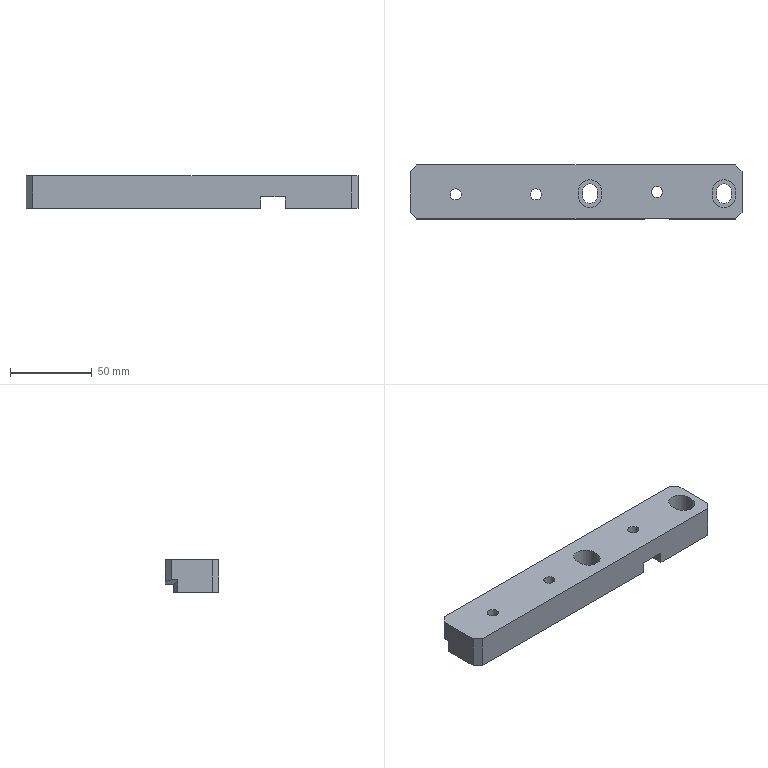Part | NX | features 20 2 | 1 solid | 43 faces | box 203 x 33 x 20 mm | volume 116194 mm3 | plane 32 | cylinder 11 | commonest cylinder face diameters 9 x4 14 x4 6.8 x3
STEP:
#1=CARTESIAN_POINT('',(39.002,-433.5,16.5));
#2=VERTEX_POINT('',#1);
#3=CARTESIAN_POINT('',(25.002,-433.5,16.5));
#4=VERTEX_POINT('',#3);
#5=CARTESIAN_POINT('',(32.002,-433.5,16.5));
#6=DIRECTION('',(0.,0.,1.));
#7=DIRECTION('',(1.,0.,0.));
#8=AXIS2_PLACEMENT_3D('',#5,#6,#7);
#9=CIRCLE('',#8,7.);
#10=EDGE_CURVE('',#2,#4,#9,.T.);
#11=ORIENTED_EDGE('',*,*,#10,.F.);
#12=CARTESIAN_POINT('',(39.002,-436.5,16.5));
#13=VERTEX_POINT('',#12);
#14=CARTESIAN_POINT('',(39.002,-450.5,16.5));
#15=DIRECTION('',(0.,1.,0.));
#16=VECTOR('',#15,1000.);
#17=LINE('',#14,#16);
#18=EDGE_CURVE('',#13,#2,#17,.T.);
#19=ORIENTED_EDGE('',*,*,#18,.F.);
#20=CARTESIAN_POINT('',(25.002,-436.5,16.5));
#21=VERTEX_POINT('',#20);
#22=CARTESIAN_POINT('',(32.002,-436.5,16.5));
#23=DIRECTION('',(0.,0.,1.));
#24=DIRECTION('',(1.,0.,0.));
#25=AXIS2_PLACEMENT_3D('',#22,#23,#24);
#26=CIRCLE('',#25,7.);
#27=EDGE_CURVE('',#21,#13,#26,.T.);
#28=ORIENTED_EDGE('',*,*,#27,.F.);
#29=CARTESIAN_POINT('',(25.002,-450.5,16.5));
#30=DIRECTION('',(0.,-1.,0.));
#31=VECTOR('',#30,1000.);
#32=LINE('',#29,#31);
#33=EDGE_CURVE('',#4,#21,#32,.T.);
#34=ORIENTED_EDGE('',*,*,#33,.F.);
#35=EDGE_LOOP('',(#11,#19,#28,#34));
#36=FACE_BOUND('',#35,.T.);
#37=CARTESIAN_POINT('',(39.002,-417.5,16.5));
#38=VERTEX_POINT('',#37);
#39=CARTESIAN_POINT('',(-155.998,-417.5,16.5));
#40=VERTEX_POINT('',#39);
#41=CARTESIAN_POINT('',(-45.998,-417.5,16.5));
#42=DIRECTION('',(-1.,0.,0.));
#43=VECTOR('',#42,1000.);
#44=LINE('',#41,#43);
#45=EDGE_CURVE('',#38,#40,#44,.T.);
#46=ORIENTED_EDGE('',*,*,#45,.T.);
#47=CARTESIAN_POINT('',(-159.998,-421.5,16.5));
#48=VERTEX_POINT('',#47);
#49=CARTESIAN_POINT('',(-159.998,-421.5,16.5));
#50=DIRECTION('',(-0.7071,-0.7071,0.));
#51=VECTOR('',#50,1000.);
#52=LINE('',#49,#51);
#53=EDGE_CURVE('',#40,#48,#52,.T.);
#54=ORIENTED_EDGE('',*,*,#53,.T.);
#55=CARTESIAN_POINT('',(-159.998,-446.5,16.5));
#56=VERTEX_POINT('',#55);
#57=CARTESIAN_POINT('',(-159.998,-417.5,16.5));
#58=DIRECTION('',(0.,-1.,0.));
#59=VECTOR('',#58,1000.);
#60=LINE('',#57,#59);
#61=EDGE_CURVE('',#48,#56,#60,.T.);
#62=ORIENTED_EDGE('',*,*,#61,.T.);
#63=CARTESIAN_POINT('',(-155.998,-450.5,16.5));
#64=VERTEX_POINT('',#63);
#65=CARTESIAN_POINT('',(-155.998,-450.5,16.5));
#66=DIRECTION('',(0.7071,-0.7071,0.));
#67=VECTOR('',#66,1000.);
#68=LINE('',#65,#67);
#69=EDGE_CURVE('',#56,#64,#68,.T.);
#70=ORIENTED_EDGE('',*,*,#69,.T.);
#71=CARTESIAN_POINT('',(39.002,-450.5,16.5));
#72=VERTEX_POINT('',#71);
#73=CARTESIAN_POINT('',(-125.998,-450.5,16.5));
#74=DIRECTION('',(1.,0.,0.));
#75=VECTOR('',#74,1000.);
#76=LINE('',#73,#75);
#77=EDGE_CURVE('',#64,#72,#76,.T.);
#78=ORIENTED_EDGE('',*,*,#77,.T.);
#79=CARTESIAN_POINT('',(43.002,-446.5,16.5));
#80=VERTEX_POINT('',#79);
#81=CARTESIAN_POINT('',(43.002,-446.5,16.5));
#82=DIRECTION('',(0.7071,0.7071,0.));
#83=VECTOR('',#82,1000.);
#84=LINE('',#81,#83);
#85=EDGE_CURVE('',#72,#80,#84,.T.);
#86=ORIENTED_EDGE('',*,*,#85,.T.);
#87=CARTESIAN_POINT('',(43.002,-421.5,16.5));
#88=VERTEX_POINT('',#87);
#89=CARTESIAN_POINT('',(43.002,-450.5,16.5));
#90=DIRECTION('',(0.,1.,0.));
#91=VECTOR('',#90,1000.);
#92=LINE('',#89,#91);
#93=EDGE_CURVE('',#80,#88,#92,.T.);
#94=ORIENTED_EDGE('',*,*,#93,.T.);
#95=CARTESIAN_POINT('',(39.002,-417.5,16.5));
#96=DIRECTION('',(-0.7071,0.7071,0.));
#97=VECTOR('',#96,1000.);
#98=LINE('',#95,#97);
#99=EDGE_CURVE('',#88,#38,#98,.T.);
#100=ORIENTED_EDGE('',*,*,#99,.T.);
#101=EDGE_LOOP('',(#46,#54,#62,#70,#78,#86,#94,#100));
#102=FACE_BOUND('',#101,.T.);
#103=CARTESIAN_POINT('',(-42.998,-436.5,16.5));
#104=VERTEX_POINT('',#103);
#105=CARTESIAN_POINT('',(-42.998,-433.5,16.5));
#106=VERTEX_POINT('',#105);
#107=CARTESIAN_POINT('',(-42.998,-450.5,16.5));
#108=DIRECTION('',(0.,1.,0.));
#109=VECTOR('',#108,1000.);
#110=LINE('',#107,#109);
#111=EDGE_CURVE('',#104,#106,#110,.T.);
#112=ORIENTED_EDGE('',*,*,#111,.F.);
#113=CARTESIAN_POINT('',(-56.998,-436.5,16.5));
#114=VERTEX_POINT('',#113);
#115=CARTESIAN_POINT('',(-49.998,-436.5,16.5));
#116=DIRECTION('',(0.,0.,1.));
#117=DIRECTION('',(1.,0.,0.));
#118=AXIS2_PLACEMENT_3D('',#115,#116,#117);
#119=CIRCLE('',#118,7.);
#120=EDGE_CURVE('',#114,#104,#119,.T.);
#121=ORIENTED_EDGE('',*,*,#120,.F.);
#122=CARTESIAN_POINT('',(-56.998,-433.5,16.5));
#123=VERTEX_POINT('',#122);
#124=CARTESIAN_POINT('',(-56.998,-450.5,16.5));
#125=DIRECTION('',(0.,-1.,0.));
#126=VECTOR('',#125,1000.);
#127=LINE('',#124,#126);
#128=EDGE_CURVE('',#123,#114,#127,.T.);
#129=ORIENTED_EDGE('',*,*,#128,.F.);
#130=CARTESIAN_POINT('',(-49.998,-433.5,16.5));
#131=DIRECTION('',(0.,0.,1.));
#132=DIRECTION('',(1.,0.,0.));
#133=AXIS2_PLACEMENT_3D('',#130,#131,#132);
#134=CIRCLE('',#133,7.);
#135=EDGE_CURVE('',#106,#123,#134,.T.);
#136=ORIENTED_EDGE('',*,*,#135,.F.);
#137=EDGE_LOOP('',(#112,#121,#129,#136));
#138=FACE_BOUND('',#137,.T.);
#139=CARTESIAN_POINT('',(-79.598,-435.5,16.5));
#140=VERTEX_POINT('',#139);
#141=CARTESIAN_POINT('',(-82.998,-435.5,16.5));
#142=DIRECTION('',(0.,0.,1.));
#143=DIRECTION('',(1.,0.,0.));
#144=AXIS2_PLACEMENT_3D('',#141,#142,#143);
#145=CIRCLE('',#144,3.4);
#146=EDGE_CURVE('',#140,#140,#145,.T.);
#147=ORIENTED_EDGE('',*,*,#146,.F.);
#148=EDGE_LOOP('',(#147));
#149=FACE_BOUND('',#148,.T.);
#150=CARTESIAN_POINT('',(-128.598,-435.5,16.5));
#151=VERTEX_POINT('',#150);
#152=CARTESIAN_POINT('',(-131.998,-435.5,16.5));
#153=DIRECTION('',(0.,0.,1.));
#154=DIRECTION('',(1.,0.,0.));
#155=AXIS2_PLACEMENT_3D('',#152,#153,#154);
#156=CIRCLE('',#155,3.4);
#157=EDGE_CURVE('',#151,#151,#156,.T.);
#158=ORIENTED_EDGE('',*,*,#157,.F.);
#159=EDGE_LOOP('',(#158));
#160=FACE_BOUND('',#159,.T.);
#161=CARTESIAN_POINT('',(-5.598,-434.,16.5));
#162=VERTEX_POINT('',#161);
#163=CARTESIAN_POINT('',(-8.998,-434.,16.5));
#164=DIRECTION('',(0.,0.,-1.));
#165=DIRECTION('',(1.,0.,0.));
#166=AXIS2_PLACEMENT_3D('',#163,#164,#165);
#167=CIRCLE('',#166,3.4);
#168=EDGE_CURVE('',#162,#162,#167,.T.);
#169=ORIENTED_EDGE('',*,*,#168,.T.);
#170=EDGE_LOOP('',(#169));
#171=FACE_BOUND('',#170,.T.);
#172=CARTESIAN_POINT('',(-45.998,-450.5,16.5));
#173=DIRECTION('',(0.,0.,1.));
#174=DIRECTION('',(-1.,0.,0.));
#175=AXIS2_PLACEMENT_3D('',#172,#173,#174);
#176=PLANE('',#175);
#177=ADVANCED_FACE('',(#36,#102,#138,#149,#160,#171),#176,.T.);
#178=CARTESIAN_POINT('',(-45.498,-433.5,1.5));
#179=VERTEX_POINT('',#178);
#180=CARTESIAN_POINT('',(-45.498,-436.5,1.5));
#181=VERTEX_POINT('',#180);
#182=CARTESIAN_POINT('',(-45.498,-432.5,1.5));
#183=DIRECTION('',(0.,-1.,0.));
#184=VECTOR('',#183,1000.);
#185=LINE('',#182,#184);
#186=EDGE_CURVE('',#179,#181,#185,.T.);
#187=ORIENTED_EDGE('',*,*,#186,.T.);
#188=CARTESIAN_POINT('',(-54.498,-436.5,1.5));
#189=VERTEX_POINT('',#188);
#190=CARTESIAN_POINT('',(-49.998,-436.5,1.5));
#191=DIRECTION('',(0.,0.,-1.));
#192=DIRECTION('',(-1.,0.,0.));
#193=AXIS2_PLACEMENT_3D('',#190,#191,#192);
#194=CIRCLE('',#193,4.5);
#195=EDGE_CURVE('',#181,#189,#194,.T.);
#196=ORIENTED_EDGE('',*,*,#195,.T.);
#197=CARTESIAN_POINT('',(-54.498,-433.5,1.5));
#198=VERTEX_POINT('',#197);
#199=CARTESIAN_POINT('',(-54.498,-439.5,1.5));
#200=DIRECTION('',(0.,1.,0.));
#201=VECTOR('',#200,1000.);
#202=LINE('',#199,#201);
#203=EDGE_CURVE('',#189,#198,#202,.T.);
#204=ORIENTED_EDGE('',*,*,#203,.T.);
#205=CARTESIAN_POINT('',(-49.998,-433.5,1.5));
#206=DIRECTION('',(0.,0.,-1.));
#207=DIRECTION('',(-1.,0.,0.));
#208=AXIS2_PLACEMENT_3D('',#205,#206,#207);
#209=CIRCLE('',#208,4.5);
#210=EDGE_CURVE('',#198,#179,#209,.T.);
#211=ORIENTED_EDGE('',*,*,#210,.T.);
#212=EDGE_LOOP('',(#187,#196,#204,#211));
#213=FACE_BOUND('',#212,.T.);
#214=CARTESIAN_POINT('',(-42.998,-433.5,1.5));
#215=VERTEX_POINT('',#214);
#216=CARTESIAN_POINT('',(-56.998,-433.5,1.5));
#217=VERTEX_POINT('',#216);
#218=CARTESIAN_POINT('',(-49.998,-433.5,1.5));
#219=DIRECTION('',(0.,0.,1.));
#220=DIRECTION('',(1.,0.,0.));
#221=AXIS2_PLACEMENT_3D('',#218,#219,#220);
#222=CIRCLE('',#221,7.);
#223=EDGE_CURVE('',#215,#217,#222,.T.);
#224=ORIENTED_EDGE('',*,*,#223,.T.);
#225=CARTESIAN_POINT('',(-56.998,-436.5,1.5));
#226=VERTEX_POINT('',#225);
#227=CARTESIAN_POINT('',(-56.998,-432.5,1.5));
#228=DIRECTION('',(0.,-1.,0.));
#229=VECTOR('',#228,1000.);
#230=LINE('',#227,#229);
#231=EDGE_CURVE('',#217,#226,#230,.T.);
#232=ORIENTED_EDGE('',*,*,#231,.T.);
#233=CARTESIAN_POINT('',(-42.998,-436.5,1.5));
#234=VERTEX_POINT('',#233);
#235=CARTESIAN_POINT('',(-49.998,-436.5,1.5));
#236=DIRECTION('',(0.,0.,1.));
#237=DIRECTION('',(1.,0.,0.));
#238=AXIS2_PLACEMENT_3D('',#235,#236,#237);
#239=CIRCLE('',#238,7.);
#240=EDGE_CURVE('',#226,#234,#239,.T.);
#241=ORIENTED_EDGE('',*,*,#240,.T.);
#242=CARTESIAN_POINT('',(-42.998,-439.5,1.5));
#243=DIRECTION('',(0.,1.,0.));
#244=VECTOR('',#243,1000.);
#245=LINE('',#242,#244);
#246=EDGE_CURVE('',#234,#215,#245,.T.);
#247=ORIENTED_EDGE('',*,*,#246,.T.);
#248=EDGE_LOOP('',(#224,#232,#241,#247));
#249=FACE_BOUND('',#248,.T.);
#250=CARTESIAN_POINT('',(-49.998,-432.5,1.5));
#251=DIRECTION('',(0.,0.,-1.));
#252=DIRECTION('',(-1.,0.,0.));
#253=AXIS2_PLACEMENT_3D('',#250,#251,#252);
#254=PLANE('',#253);
#255=ADVANCED_FACE('',(#213,#249),#254,.F.);
#256=CARTESIAN_POINT('',(27.502,-436.5,1.5));
#257=VERTEX_POINT('',#256);
#258=CARTESIAN_POINT('',(27.502,-433.5,1.5));
#259=VERTEX_POINT('',#258);
#260=CARTESIAN_POINT('',(27.502,-432.5,1.5));
#261=DIRECTION('',(0.,1.,0.));
#262=VECTOR('',#261,1000.);
#263=LINE('',#260,#262);
#264=EDGE_CURVE('',#257,#259,#263,.T.);
#265=ORIENTED_EDGE('',*,*,#264,.T.);
#266=CARTESIAN_POINT('',(36.502,-433.5,1.5));
#267=VERTEX_POINT('',#266);
#268=CARTESIAN_POINT('',(32.002,-433.5,1.5));
#269=DIRECTION('',(0.,0.,-1.));
#270=DIRECTION('',(1.,0.,0.));
#271=AXIS2_PLACEMENT_3D('',#268,#269,#270);
#272=CIRCLE('',#271,4.5);
#273=EDGE_CURVE('',#259,#267,#272,.T.);
#274=ORIENTED_EDGE('',*,*,#273,.T.);
#275=CARTESIAN_POINT('',(36.502,-436.5,1.5));
#276=VERTEX_POINT('',#275);
#277=CARTESIAN_POINT('',(36.502,-439.5,1.5));
#278=DIRECTION('',(0.,-1.,0.));
#279=VECTOR('',#278,1000.);
#280=LINE('',#277,#279);
#281=EDGE_CURVE('',#267,#276,#280,.T.);
#282=ORIENTED_EDGE('',*,*,#281,.T.);
#283=CARTESIAN_POINT('',(32.002,-436.5,1.5));
#284=DIRECTION('',(0.,0.,-1.));
#285=DIRECTION('',(1.,0.,0.));
#286=AXIS2_PLACEMENT_3D('',#283,#284,#285);
#287=CIRCLE('',#286,4.5);
#288=EDGE_CURVE('',#276,#257,#287,.T.);
#289=ORIENTED_EDGE('',*,*,#288,.T.);
#290=EDGE_LOOP('',(#265,#274,#282,#289));
#291=FACE_BOUND('',#290,.T.);
#292=CARTESIAN_POINT('',(39.002,-433.5,1.5));
#293=VERTEX_POINT('',#292);
#294=CARTESIAN_POINT('',(25.002,-433.5,1.5));
#295=VERTEX_POINT('',#294);
#296=CARTESIAN_POINT('',(32.002,-433.5,1.5));
#297=DIRECTION('',(0.,0.,1.));
#298=DIRECTION('',(-1.,0.,0.));
#299=AXIS2_PLACEMENT_3D('',#296,#297,#298);
#300=CIRCLE('',#299,7.);
#301=EDGE_CURVE('',#293,#295,#300,.T.);
#302=ORIENTED_EDGE('',*,*,#301,.T.);
#303=CARTESIAN_POINT('',(25.002,-436.5,1.5));
#304=VERTEX_POINT('',#303);
#305=CARTESIAN_POINT('',(25.002,-439.5,1.5));
#306=DIRECTION('',(0.,-1.,0.));
#307=VECTOR('',#306,1000.);
#308=LINE('',#305,#307);
#309=EDGE_CURVE('',#295,#304,#308,.T.);
#310=ORIENTED_EDGE('',*,*,#309,.T.);
#311=CARTESIAN_POINT('',(39.002,-436.5,1.5));
#312=VERTEX_POINT('',#311);
#313=CARTESIAN_POINT('',(32.002,-436.5,1.5));
#314=DIRECTION('',(0.,0.,1.));
#315=DIRECTION('',(-1.,0.,0.));
#316=AXIS2_PLACEMENT_3D('',#313,#314,#315);
#317=CIRCLE('',#316,7.);
#318=EDGE_CURVE('',#304,#312,#317,.T.);
#319=ORIENTED_EDGE('',*,*,#318,.T.);
#320=CARTESIAN_POINT('',(39.002,-432.5,1.5));
#321=DIRECTION('',(0.,1.,0.));
#322=VECTOR('',#321,1000.);
#323=LINE('',#320,#322);
#324=EDGE_CURVE('',#312,#293,#323,.T.);
#325=ORIENTED_EDGE('',*,*,#324,.T.);
#326=EDGE_LOOP('',(#302,#310,#319,#325));
#327=FACE_BOUND('',#326,.T.);
#328=CARTESIAN_POINT('',(32.002,-432.5,1.5));
#329=DIRECTION('',(0.,0.,-1.));
#330=DIRECTION('',(1.,0.,0.));
#331=AXIS2_PLACEMENT_3D('',#328,#329,#330);
#332=PLANE('',#331);
#333=ADVANCED_FACE('',(#291,#327),#332,.F.);
#334=CARTESIAN_POINT('',(-149.999,-422.5,-3.5));
#335=VERTEX_POINT('',#334);
#336=CARTESIAN_POINT('',(-159.998,-425.179,-3.5));
#337=VERTEX_POINT('',#336);
#338=CARTESIAN_POINT('',(-149.999,-422.5,-3.5));
#339=DIRECTION('',(-0.9659,-0.2588,0.));
#340=VECTOR('',#339,1000.);
#341=LINE('',#338,#340);
#342=EDGE_CURVE('',#335,#337,#341,.T.);
#343=ORIENTED_EDGE('',*,*,#342,.T.);
#344=CARTESIAN_POINT('',(-159.998,-425.179,4.179));
#345=VERTEX_POINT('',#344);
#346=CARTESIAN_POINT('',(-159.998,-425.179,3.5));
#347=DIRECTION('',(0.,0.,-1.));
#348=VECTOR('',#347,1000.);
#349=LINE('',#346,#348);
#350=EDGE_CURVE('',#345,#337,#349,.T.);
#351=ORIENTED_EDGE('',*,*,#350,.F.);
#352=CARTESIAN_POINT('',(-149.999,-422.5,1.5));
#353=VERTEX_POINT('',#352);
#354=CARTESIAN_POINT('',(-149.999,-422.5,1.5));
#355=DIRECTION('',(0.9351,0.2506,-0.2506));
#356=VECTOR('',#355,1000.);
#357=LINE('',#354,#356);
#358=EDGE_CURVE('',#345,#353,#357,.T.);
#359=ORIENTED_EDGE('',*,*,#358,.T.);
#360=CARTESIAN_POINT('',(-149.999,-422.5,3.5));
#361=DIRECTION('',(0.,0.,1.));
#362=VECTOR('',#361,1000.);
#363=LINE('',#360,#362);
#364=EDGE_CURVE('',#335,#353,#363,.T.);
#365=ORIENTED_EDGE('',*,*,#364,.F.);
#366=EDGE_LOOP('',(#343,#351,#359,#365));
#367=FACE_BOUND('',#366,.T.);
#368=CARTESIAN_POINT('',(-149.999,-422.5,3.5));
#369=DIRECTION('',(0.2588,-0.9659,0.));
#370=DIRECTION('',(0.9659,0.2588,0.));
#371=AXIS2_PLACEMENT_3D('',#368,#369,#370);
#372=PLANE('',#371);
#373=ADVANCED_FACE('',(#367),#372,.F.);
#374=CARTESIAN_POINT('',(-16.498,-422.5,-3.5));
#375=VERTEX_POINT('',#374);
#376=CARTESIAN_POINT('',(-16.498,-422.5,1.5));
#377=VERTEX_POINT('',#376);
#378=CARTESIAN_POINT('',(-16.498,-422.5,-9.5));
#379=DIRECTION('',(0.,0.,1.));
#380=VECTOR('',#379,1000.);
#381=LINE('',#378,#380);
#382=EDGE_CURVE('',#375,#377,#381,.T.);
#383=ORIENTED_EDGE('',*,*,#382,.F.);
#384=CARTESIAN_POINT('',(-46.,-422.5,-3.5));
#385=DIRECTION('',(-1.,0.,0.));
#386=VECTOR('',#385,1000.);
#387=LINE('',#384,#386);
#388=EDGE_CURVE('',#375,#335,#387,.T.);
#389=ORIENTED_EDGE('',*,*,#388,.T.);
#390=ORIENTED_EDGE('',*,*,#364,.T.);
#391=CARTESIAN_POINT('',(-149.998,-422.5,1.5));
#392=VERTEX_POINT('',#391);
#393=CARTESIAN_POINT('',(-94.019,-422.5,-13.5));
#394=DIRECTION('',(0.9659,0.,-0.2588));
#395=VECTOR('',#394,1000.);
#396=LINE('',#393,#395);
#397=EDGE_CURVE('',#353,#392,#396,.T.);
#398=ORIENTED_EDGE('',*,*,#397,.T.);
#399=CARTESIAN_POINT('',(-56.,-422.5,1.5));
#400=DIRECTION('',(1.,0.,0.));
#401=VECTOR('',#400,1000.);
#402=LINE('',#399,#401);
#403=EDGE_CURVE('',#392,#377,#402,.T.);
#404=ORIENTED_EDGE('',*,*,#403,.T.);
#405=EDGE_LOOP('',(#383,#389,#390,#398,#404));
#406=FACE_BOUND('',#405,.T.);
#407=CARTESIAN_POINT('',(-56.,-422.5,3.5));
#408=DIRECTION('',(0.,-1.,0.));
#409=DIRECTION('',(0.,0.,1.));
#410=AXIS2_PLACEMENT_3D('',#407,#408,#409);
#411=PLANE('',#410);
#412=ADVANCED_FACE('',(#406),#411,.F.);
#413=ORIENTED_EDGE('',*,*,#195,.F.);
#414=CARTESIAN_POINT('',(-45.498,-436.5,-3.5));
#415=VERTEX_POINT('',#414);
#416=CARTESIAN_POINT('',(-45.498,-436.5,42.5));
#417=DIRECTION('',(0.,0.,-1.));
#418=VECTOR('',#417,1000.);
#419=LINE('',#416,#418);
#420=EDGE_CURVE('',#181,#415,#419,.T.);
#421=ORIENTED_EDGE('',*,*,#420,.T.);
#422=CARTESIAN_POINT('',(-54.498,-436.5,-3.5));
#423=VERTEX_POINT('',#422);
#424=CARTESIAN_POINT('',(-49.998,-436.5,-3.5));
#425=DIRECTION('',(0.,0.,-1.));
#426=DIRECTION('',(1.,0.,0.));
#427=AXIS2_PLACEMENT_3D('',#424,#425,#426);
#428=CIRCLE('',#427,4.5);
#429=EDGE_CURVE('',#415,#423,#428,.T.);
#430=ORIENTED_EDGE('',*,*,#429,.T.);
#431=CARTESIAN_POINT('',(-54.498,-436.5,42.5));
#432=DIRECTION('',(0.,0.,-1.));
#433=VECTOR('',#432,1000.);
#434=LINE('',#431,#433);
#435=EDGE_CURVE('',#189,#423,#434,.T.);
#436=ORIENTED_EDGE('',*,*,#435,.F.);
#437=EDGE_LOOP('',(#413,#421,#430,#436));
#438=FACE_BOUND('',#437,.T.);
#439=CARTESIAN_POINT('',(-49.998,-436.5,42.5));
#440=DIRECTION('',(0.,0.,-1.));
#441=DIRECTION('',(-1.,0.,0.));
#442=AXIS2_PLACEMENT_3D('',#439,#440,#441);
#443=CYLINDRICAL_SURFACE('',#442,4.5);
#444=ADVANCED_FACE('',(#438),#443,.F.);
#445=ORIENTED_EDGE('',*,*,#203,.F.);
#446=ORIENTED_EDGE('',*,*,#435,.T.);
#447=CARTESIAN_POINT('',(-54.498,-433.5,-3.5));
#448=VERTEX_POINT('',#447);
#449=CARTESIAN_POINT('',(-54.498,-450.5,-3.5));
#450=DIRECTION('',(0.,1.,0.));
#451=VECTOR('',#450,1000.);
#452=LINE('',#449,#451);
#453=EDGE_CURVE('',#423,#448,#452,.T.);
#454=ORIENTED_EDGE('',*,*,#453,.T.);
#455=CARTESIAN_POINT('',(-54.498,-433.5,42.5));
#456=DIRECTION('',(0.,0.,-1.));
#457=VECTOR('',#456,1000.);
#458=LINE('',#455,#457);
#459=EDGE_CURVE('',#198,#448,#458,.T.);
#460=ORIENTED_EDGE('',*,*,#459,.F.);
#461=EDGE_LOOP('',(#445,#446,#454,#460));
#462=FACE_BOUND('',#461,.T.);
#463=CARTESIAN_POINT('',(-54.498,-439.5,42.5));
#464=DIRECTION('',(1.,0.,0.));
#465=DIRECTION('',(0.,0.,-1.));
#466=AXIS2_PLACEMENT_3D('',#463,#464,#465);
#467=PLANE('',#466);
#468=ADVANCED_FACE('',(#462),#467,.T.);
#469=ORIENTED_EDGE('',*,*,#210,.F.);
#470=ORIENTED_EDGE('',*,*,#459,.T.);
#471=CARTESIAN_POINT('',(-45.498,-433.5,-3.5));
#472=VERTEX_POINT('',#471);
#473=CARTESIAN_POINT('',(-49.998,-433.5,-3.5));
#474=DIRECTION('',(0.,0.,-1.));
#475=DIRECTION('',(1.,0.,0.));
#476=AXIS2_PLACEMENT_3D('',#473,#474,#475);
#477=CIRCLE('',#476,4.5);
#478=EDGE_CURVE('',#448,#472,#477,.T.);
#479=ORIENTED_EDGE('',*,*,#478,.T.);
#480=CARTESIAN_POINT('',(-45.498,-433.5,42.5));
#481=DIRECTION('',(0.,0.,-1.));
#482=VECTOR('',#481,1000.);
#483=LINE('',#480,#482);
#484=EDGE_CURVE('',#179,#472,#483,.T.);
#485=ORIENTED_EDGE('',*,*,#484,.F.);
#486=EDGE_LOOP('',(#469,#470,#479,#485));
#487=FACE_BOUND('',#486,.T.);
#488=CARTESIAN_POINT('',(-49.998,-433.5,42.5));
#489=DIRECTION('',(0.,0.,-1.));
#490=DIRECTION('',(-1.,0.,0.));
#491=AXIS2_PLACEMENT_3D('',#488,#489,#490);
#492=CYLINDRICAL_SURFACE('',#491,4.5);
#493=ADVANCED_FACE('',(#487),#492,.F.);
#494=ORIENTED_EDGE('',*,*,#186,.F.);
#495=ORIENTED_EDGE('',*,*,#484,.T.);
#496=CARTESIAN_POINT('',(-45.498,-450.5,-3.5));
#497=DIRECTION('',(0.,-1.,0.));
#498=VECTOR('',#497,1000.);
#499=LINE('',#496,#498);
#500=EDGE_CURVE('',#472,#415,#499,.T.);
#501=ORIENTED_EDGE('',*,*,#500,.T.);
#502=ORIENTED_EDGE('',*,*,#420,.F.);
#503=EDGE_LOOP('',(#494,#495,#501,#502));
#504=FACE_BOUND('',#503,.T.);
#505=CARTESIAN_POINT('',(-45.498,-432.5,42.5));
#506=DIRECTION('',(-1.,0.,0.));
#507=DIRECTION('',(0.,0.,1.));
#508=AXIS2_PLACEMENT_3D('',#505,#506,#507);
#509=PLANE('',#508);
#510=ADVANCED_FACE('',(#504),#509,.T.);
#511=CARTESIAN_POINT('',(-128.598,-435.5,-3.5));
#512=VERTEX_POINT('',#511);
#513=CARTESIAN_POINT('',(-131.998,-435.5,-3.5));
#514=DIRECTION('',(0.,0.,1.));
#515=DIRECTION('',(1.,0.,0.));
#516=AXIS2_PLACEMENT_3D('',#513,#514,#515);
#517=CIRCLE('',#516,3.4);
#518=EDGE_CURVE('',#512,#512,#517,.T.);
#519=ORIENTED_EDGE('',*,*,#518,.F.);
#520=EDGE_LOOP('',(#519));
#521=FACE_BOUND('',#520,.T.);
#522=ORIENTED_EDGE('',*,*,#157,.T.);
#523=EDGE_LOOP('',(#522));
#524=FACE_BOUND('',#523,.T.);
#525=CARTESIAN_POINT('',(-131.998,-435.5,-3.5));
#526=DIRECTION('',(0.,0.,1.));
#527=DIRECTION('',(1.,0.,0.));
#528=AXIS2_PLACEMENT_3D('',#525,#526,#527);
#529=CYLINDRICAL_SURFACE('',#528,3.4);
#530=ADVANCED_FACE('',(#521,#524),#529,.F.);
#531=CARTESIAN_POINT('',(-79.598,-435.5,-3.5));
#532=VERTEX_POINT('',#531);
#533=CARTESIAN_POINT('',(-82.998,-435.5,-3.5));
#534=DIRECTION('',(0.,0.,1.));
#535=DIRECTION('',(1.,0.,0.));
#536=AXIS2_PLACEMENT_3D('',#533,#534,#535);
#537=CIRCLE('',#536,3.4);
#538=EDGE_CURVE('',#532,#532,#537,.T.);
#539=ORIENTED_EDGE('',*,*,#538,.F.);
#540=EDGE_LOOP('',(#539));
#541=FACE_BOUND('',#540,.T.);
#542=ORIENTED_EDGE('',*,*,#146,.T.);
#543=EDGE_LOOP('',(#542));
#544=FACE_BOUND('',#543,.T.);
#545=CARTESIAN_POINT('',(-82.998,-435.5,-3.5));
#546=DIRECTION('',(0.,0.,1.));
#547=DIRECTION('',(1.,0.,0.));
#548=AXIS2_PLACEMENT_3D('',#545,#546,#547);
#549=CYLINDRICAL_SURFACE('',#548,3.4);
#550=ADVANCED_FACE('',(#541,#544),#549,.F.);
#551=ORIENTED_EDGE('',*,*,#33,.T.);
#552=CARTESIAN_POINT('',(25.002,-436.5,42.5));
#553=DIRECTION('',(0.,0.,1.));
#554=VECTOR('',#553,1000.);
#555=LINE('',#552,#554);
#556=EDGE_CURVE('',#304,#21,#555,.T.);
#557=ORIENTED_EDGE('',*,*,#556,.F.);
#558=ORIENTED_EDGE('',*,*,#309,.F.);
#559=CARTESIAN_POINT('',(25.002,-433.5,42.5));
#560=DIRECTION('',(0.,0.,1.));
#561=VECTOR('',#560,1000.);
#562=LINE('',#559,#561);
#563=EDGE_CURVE('',#295,#4,#562,.T.);
#564=ORIENTED_EDGE('',*,*,#563,.T.);
#565=EDGE_LOOP('',(#551,#557,#558,#564));
#566=FACE_BOUND('',#565,.T.);
#567=CARTESIAN_POINT('',(25.002,-439.5,42.5));
#568=DIRECTION('',(-1.,0.,0.));
#569=DIRECTION('',(0.,0.,-1.));
#570=AXIS2_PLACEMENT_3D('',#567,#568,#569);
#571=PLANE('',#570);
#572=ADVANCED_FACE('',(#566),#571,.F.);
#573=ORIENTED_EDGE('',*,*,#27,.T.);
#574=CARTESIAN_POINT('',(39.002,-436.5,42.5));
#575=DIRECTION('',(0.,0.,1.));
#576=VECTOR('',#575,1000.);
#577=LINE('',#574,#576);
#578=EDGE_CURVE('',#312,#13,#577,.T.);
#579=ORIENTED_EDGE('',*,*,#578,.F.);
#580=ORIENTED_EDGE('',*,*,#318,.F.);
#581=ORIENTED_EDGE('',*,*,#556,.T.);
#582=EDGE_LOOP('',(#573,#579,#580,#581));
#583=FACE_BOUND('',#582,.T.);
#584=CARTESIAN_POINT('',(32.002,-436.5,42.5));
#585=DIRECTION('',(0.,0.,-1.));
#586=DIRECTION('',(1.,0.,0.));
#587=AXIS2_PLACEMENT_3D('',#584,#585,#586);
#588=CYLINDRICAL_SURFACE('',#587,7.);
#589=ADVANCED_FACE('',(#583),#588,.F.);
#590=ORIENTED_EDGE('',*,*,#18,.T.);
#591=CARTESIAN_POINT('',(39.002,-433.5,42.5));
#592=DIRECTION('',(0.,0.,1.));
#593=VECTOR('',#592,1000.);
#594=LINE('',#591,#593);
#595=EDGE_CURVE('',#293,#2,#594,.T.);
#596=ORIENTED_EDGE('',*,*,#595,.F.);
#597=ORIENTED_EDGE('',*,*,#324,.F.);
#598=ORIENTED_EDGE('',*,*,#578,.T.);
#599=EDGE_LOOP('',(#590,#596,#597,#598));
#600=FACE_BOUND('',#599,.T.);
#601=CARTESIAN_POINT('',(39.002,-432.5,42.5));
#602=DIRECTION('',(1.,0.,0.));
#603=DIRECTION('',(0.,0.,1.));
#604=AXIS2_PLACEMENT_3D('',#601,#602,#603);
#605=PLANE('',#604);
#606=ADVANCED_FACE('',(#600),#605,.F.);
#607=ORIENTED_EDGE('',*,*,#10,.T.);
#608=ORIENTED_EDGE('',*,*,#563,.F.);
#609=ORIENTED_EDGE('',*,*,#301,.F.);
#610=ORIENTED_EDGE('',*,*,#595,.T.);
#611=EDGE_LOOP('',(#607,#608,#609,#610));
#612=FACE_BOUND('',#611,.T.);
#613=CARTESIAN_POINT('',(32.002,-433.5,42.5));
#614=DIRECTION('',(0.,0.,-1.));
#615=DIRECTION('',(1.,0.,0.));
#616=AXIS2_PLACEMENT_3D('',#613,#614,#615);
#617=CYLINDRICAL_SURFACE('',#616,7.);
#618=ADVANCED_FACE('',(#612),#617,.F.);
#619=CARTESIAN_POINT('',(-159.998,-446.5,-3.5));
#620=VERTEX_POINT('',#619);
#621=CARTESIAN_POINT('',(-159.998,-446.5,11.5));
#622=DIRECTION('',(0.,0.,1.));
#623=VECTOR('',#622,1000.);
#624=LINE('',#621,#623);
#625=EDGE_CURVE('',#620,#56,#624,.T.);
#626=ORIENTED_EDGE('',*,*,#625,.T.);
#627=ORIENTED_EDGE('',*,*,#61,.F.);
#628=CARTESIAN_POINT('',(-159.998,-421.5,4.179));
#629=VERTEX_POINT('',#628);
#630=CARTESIAN_POINT('',(-159.998,-421.5,11.5));
#631=DIRECTION('',(0.,0.,-1.));
#632=VECTOR('',#631,1000.);
#633=LINE('',#630,#632);
#634=EDGE_CURVE('',#48,#629,#633,.T.);
#635=ORIENTED_EDGE('',*,*,#634,.T.);
#636=CARTESIAN_POINT('',(-159.998,-425.179,4.179));
#637=DIRECTION('',(0.,-1.,0.));
#638=VECTOR('',#637,1000.);
#639=LINE('',#636,#638);
#640=EDGE_CURVE('',#629,#345,#639,.T.);
#641=ORIENTED_EDGE('',*,*,#640,.T.);
#642=ORIENTED_EDGE('',*,*,#350,.T.);
#643=CARTESIAN_POINT('',(-159.998,-417.5,-3.5));
#644=DIRECTION('',(0.,-1.,0.));
#645=VECTOR('',#644,1000.);
#646=LINE('',#643,#645);
#647=EDGE_CURVE('',#337,#620,#646,.T.);
#648=ORIENTED_EDGE('',*,*,#647,.T.);
#649=EDGE_LOOP('',(#626,#627,#635,#641,#642,#648));
#650=FACE_BOUND('',#649,.T.);
#651=CARTESIAN_POINT('',(-159.998,-417.5,11.5));
#652=DIRECTION('',(1.,0.,0.));
#653=DIRECTION('',(0.,0.,1.));
#654=AXIS2_PLACEMENT_3D('',#651,#652,#653);
#655=PLANE('',#654);
#656=ADVANCED_FACE('',(#650),#655,.F.);
#657=ORIENTED_EDGE('',*,*,#135,.T.);
#658=CARTESIAN_POINT('',(-56.998,-433.5,42.5));
#659=DIRECTION('',(0.,0.,-1.));
#660=VECTOR('',#659,1000.);
#661=LINE('',#658,#660);
#662=EDGE_CURVE('',#123,#217,#661,.T.);
#663=ORIENTED_EDGE('',*,*,#662,.T.);
#664=ORIENTED_EDGE('',*,*,#223,.F.);
#665=CARTESIAN_POINT('',(-42.998,-433.5,42.5));
#666=DIRECTION('',(0.,0.,-1.));
#667=VECTOR('',#666,1000.);
#668=LINE('',#665,#667);
#669=EDGE_CURVE('',#106,#215,#668,.T.);
#670=ORIENTED_EDGE('',*,*,#669,.F.);
#671=EDGE_LOOP('',(#657,#663,#664,#670));
#672=FACE_BOUND('',#671,.T.);
#673=CARTESIAN_POINT('',(-49.998,-433.5,42.5));
#674=DIRECTION('',(0.,0.,-1.));
#675=DIRECTION('',(-1.,0.,0.));
#676=AXIS2_PLACEMENT_3D('',#673,#674,#675);
#677=CYLINDRICAL_SURFACE('',#676,7.);
#678=ADVANCED_FACE('',(#672),#677,.F.);
#679=ORIENTED_EDGE('',*,*,#128,.T.);
#680=CARTESIAN_POINT('',(-56.998,-436.5,42.5));
#681=DIRECTION('',(0.,0.,-1.));
#682=VECTOR('',#681,1000.);
#683=LINE('',#680,#682);
#684=EDGE_CURVE('',#114,#226,#683,.T.);
#685=ORIENTED_EDGE('',*,*,#684,.T.);
#686=ORIENTED_EDGE('',*,*,#231,.F.);
#687=ORIENTED_EDGE('',*,*,#662,.F.);
#688=EDGE_LOOP('',(#679,#685,#686,#687));
#689=FACE_BOUND('',#688,.T.);
#690=CARTESIAN_POINT('',(-56.998,-432.5,42.5));
#691=DIRECTION('',(-1.,0.,0.));
#692=DIRECTION('',(0.,0.,1.));
#693=AXIS2_PLACEMENT_3D('',#690,#691,#692);
#694=PLANE('',#693);
#695=ADVANCED_FACE('',(#689),#694,.F.);
#696=ORIENTED_EDGE('',*,*,#120,.T.);
#697=CARTESIAN_POINT('',(-42.998,-436.5,42.5));
#698=DIRECTION('',(0.,0.,-1.));
#699=VECTOR('',#698,1000.);
#700=LINE('',#697,#699);
#701=EDGE_CURVE('',#104,#234,#700,.T.);
#702=ORIENTED_EDGE('',*,*,#701,.T.);
#703=ORIENTED_EDGE('',*,*,#240,.F.);
#704=ORIENTED_EDGE('',*,*,#684,.F.);
#705=EDGE_LOOP('',(#696,#702,#703,#704));
#706=FACE_BOUND('',#705,.T.);
#707=CARTESIAN_POINT('',(-49.998,-436.5,42.5));
#708=DIRECTION('',(0.,0.,-1.));
#709=DIRECTION('',(-1.,0.,0.));
#710=AXIS2_PLACEMENT_3D('',#707,#708,#709);
#711=CYLINDRICAL_SURFACE('',#710,7.);
#712=ADVANCED_FACE('',(#706),#711,.F.);
#713=ORIENTED_EDGE('',*,*,#111,.T.);
#714=ORIENTED_EDGE('',*,*,#669,.T.);
#715=ORIENTED_EDGE('',*,*,#246,.F.);
#716=ORIENTED_EDGE('',*,*,#701,.F.);
#717=EDGE_LOOP('',(#713,#714,#715,#716));
#718=FACE_BOUND('',#717,.T.);
#719=CARTESIAN_POINT('',(-42.998,-439.5,42.5));
#720=DIRECTION('',(1.,0.,0.));
#721=DIRECTION('',(0.,0.,-1.));
#722=AXIS2_PLACEMENT_3D('',#719,#720,#721);
#723=PLANE('',#722);
#724=ADVANCED_FACE('',(#718),#723,.F.);
#725=CARTESIAN_POINT('',(-1.498,-422.5,1.5));
#726=VERTEX_POINT('',#725);
#727=CARTESIAN_POINT('',(29.268,-422.5,1.5));
#728=VERTEX_POINT('',#727);
#729=CARTESIAN_POINT('',(-56.,-422.5,1.5));
#730=DIRECTION('',(1.,0.,0.));
#731=VECTOR('',#730,1000.);
#732=LINE('',#729,#731);
#733=EDGE_CURVE('',#726,#728,#732,.T.);
#734=ORIENTED_EDGE('',*,*,#733,.T.);
#735=CARTESIAN_POINT('',(29.268,-422.5,-3.5));
#736=VERTEX_POINT('',#735);
#737=CARTESIAN_POINT('',(29.268,-422.5,3.5));
#738=DIRECTION('',(0.,0.,1.));
#739=VECTOR('',#738,1000.);
#740=LINE('',#737,#739);
#741=EDGE_CURVE('',#736,#728,#740,.T.);
#742=ORIENTED_EDGE('',*,*,#741,.F.);
#743=CARTESIAN_POINT('',(-1.498,-422.5,-3.5));
#744=VERTEX_POINT('',#743);
#745=CARTESIAN_POINT('',(-46.,-422.5,-3.5));
#746=DIRECTION('',(-1.,0.,0.));
#747=VECTOR('',#746,1000.);
#748=LINE('',#745,#747);
#749=EDGE_CURVE('',#736,#744,#748,.T.);
#750=ORIENTED_EDGE('',*,*,#749,.T.);
#751=CARTESIAN_POINT('',(-1.498,-422.5,-9.5));
#752=DIRECTION('',(0.,0.,-1.));
#753=VECTOR('',#752,1000.);
#754=LINE('',#751,#753);
#755=EDGE_CURVE('',#726,#744,#754,.T.);
#756=ORIENTED_EDGE('',*,*,#755,.F.);
#757=EDGE_LOOP('',(#734,#742,#750,#756));
#758=FACE_BOUND('',#757,.T.);
#759=CARTESIAN_POINT('',(-56.,-422.5,3.5));
#760=DIRECTION('',(0.,-1.,0.));
#761=DIRECTION('',(0.,0.,1.));
#762=AXIS2_PLACEMENT_3D('',#759,#760,#761);
#763=PLANE('',#762);
#764=ADVANCED_FACE('',(#758),#763,.F.);
#765=CARTESIAN_POINT('',(43.002,-446.5,-3.5));
#766=VERTEX_POINT('',#765);
#767=CARTESIAN_POINT('',(43.002,-426.18,-3.5));
#768=VERTEX_POINT('',#767);
#769=CARTESIAN_POINT('',(43.002,-450.5,-3.5));
#770=DIRECTION('',(0.,1.,0.));
#771=VECTOR('',#770,1000.);
#772=LINE('',#769,#771);
#773=EDGE_CURVE('',#766,#768,#772,.T.);
#774=ORIENTED_EDGE('',*,*,#773,.T.);
#775=CARTESIAN_POINT('',(43.002,-426.18,4.179));
#776=VERTEX_POINT('',#775);
#777=CARTESIAN_POINT('',(43.002,-426.18,3.5));
#778=DIRECTION('',(0.,0.,-1.));
#779=VECTOR('',#778,1000.);
#780=LINE('',#777,#779);
#781=EDGE_CURVE('',#776,#768,#780,.T.);
#782=ORIENTED_EDGE('',*,*,#781,.F.);
#783=CARTESIAN_POINT('',(43.002,-421.5,4.179));
#784=VERTEX_POINT('',#783);
#785=CARTESIAN_POINT('',(43.002,-417.5,4.179));
#786=DIRECTION('',(0.,1.,0.));
#787=VECTOR('',#786,1000.);
#788=LINE('',#785,#787);
#789=EDGE_CURVE('',#776,#784,#788,.T.);
#790=ORIENTED_EDGE('',*,*,#789,.T.);
#791=CARTESIAN_POINT('',(43.002,-421.5,11.5));
#792=DIRECTION('',(0.,0.,1.));
#793=VECTOR('',#792,1000.);
#794=LINE('',#791,#793);
#795=EDGE_CURVE('',#784,#88,#794,.T.);
#796=ORIENTED_EDGE('',*,*,#795,.T.);
#797=ORIENTED_EDGE('',*,*,#93,.F.);
#798=CARTESIAN_POINT('',(43.002,-446.5,11.5));
#799=DIRECTION('',(0.,0.,-1.));
#800=VECTOR('',#799,1000.);
#801=LINE('',#798,#800);
#802=EDGE_CURVE('',#80,#766,#801,.T.);
#803=ORIENTED_EDGE('',*,*,#802,.T.);
#804=EDGE_LOOP('',(#774,#782,#790,#796,#797,#803));
#805=FACE_BOUND('',#804,.T.);
#806=CARTESIAN_POINT('',(43.002,-450.5,11.5));
#807=DIRECTION('',(-1.,0.,0.));
#808=DIRECTION('',(0.,0.,-1.));
#809=AXIS2_PLACEMENT_3D('',#806,#807,#808);
#810=PLANE('',#809);
#811=ADVANCED_FACE('',(#805),#810,.F.);
#812=CARTESIAN_POINT('',(33.002,-423.5,1.5));
#813=VERTEX_POINT('',#812);
#814=CARTESIAN_POINT('',(43.002,-426.18,1.5));
#815=DIRECTION('',(0.9659,-0.2588,0.));
#816=VECTOR('',#815,1000.);
#817=LINE('',#814,#816);
#818=EDGE_CURVE('',#728,#813,#817,.T.);
#819=ORIENTED_EDGE('',*,*,#818,.T.);
#820=CARTESIAN_POINT('',(42.374,-426.012,4.011));
#821=DIRECTION('',(0.9351,-0.2506,0.2506));
#822=VECTOR('',#821,1000.);
#823=LINE('',#820,#822);
#824=EDGE_CURVE('',#813,#776,#823,.T.);
#825=ORIENTED_EDGE('',*,*,#824,.T.);
#826=ORIENTED_EDGE('',*,*,#781,.T.);
#827=CARTESIAN_POINT('',(43.002,-426.18,-3.5));
#828=DIRECTION('',(-0.9659,0.2588,0.));
#829=VECTOR('',#828,1000.);
#830=LINE('',#827,#829);
#831=EDGE_CURVE('',#768,#736,#830,.T.);
#832=ORIENTED_EDGE('',*,*,#831,.T.);
#833=ORIENTED_EDGE('',*,*,#741,.T.);
#834=EDGE_LOOP('',(#819,#825,#826,#832,#833));
#835=FACE_BOUND('',#834,.T.);
#836=CARTESIAN_POINT('',(43.002,-426.18,3.5));
#837=DIRECTION('',(-0.2588,-0.9659,0.));
#838=DIRECTION('',(0.9659,-0.2588,0.));
#839=AXIS2_PLACEMENT_3D('',#836,#837,#838);
#840=PLANE('',#839);
#841=ADVANCED_FACE('',(#835),#840,.F.);
#842=ORIENTED_EDGE('',*,*,#273,.F.);
#843=CARTESIAN_POINT('',(27.502,-433.5,-3.5));
#844=VERTEX_POINT('',#843);
#845=CARTESIAN_POINT('',(27.502,-433.5,42.5));
#846=DIRECTION('',(0.,0.,1.));
#847=VECTOR('',#846,1000.);
#848=LINE('',#845,#847);
#849=EDGE_CURVE('',#844,#259,#848,.T.);
#850=ORIENTED_EDGE('',*,*,#849,.F.);
#851=CARTESIAN_POINT('',(36.502,-433.5,-3.5));
#852=VERTEX_POINT('',#851);
#853=CARTESIAN_POINT('',(32.002,-433.5,-3.5));
#854=DIRECTION('',(0.,0.,1.));
#855=DIRECTION('',(1.,0.,0.));
#856=AXIS2_PLACEMENT_3D('',#853,#854,#855);
#857=CIRCLE('',#856,4.5);
#858=EDGE_CURVE('',#852,#844,#857,.T.);
#859=ORIENTED_EDGE('',*,*,#858,.F.);
#860=CARTESIAN_POINT('',(36.502,-433.5,42.5));
#861=DIRECTION('',(0.,0.,1.));
#862=VECTOR('',#861,1000.);
#863=LINE('',#860,#862);
#864=EDGE_CURVE('',#852,#267,#863,.T.);
#865=ORIENTED_EDGE('',*,*,#864,.T.);
#866=EDGE_LOOP('',(#842,#850,#859,#865));
#867=FACE_BOUND('',#866,.T.);
#868=CARTESIAN_POINT('',(32.002,-433.5,42.5));
#869=DIRECTION('',(0.,0.,-1.));
#870=DIRECTION('',(1.,0.,0.));
#871=AXIS2_PLACEMENT_3D('',#868,#869,#870);
#872=CYLINDRICAL_SURFACE('',#871,4.5);
#873=ADVANCED_FACE('',(#867),#872,.F.);
#874=ORIENTED_EDGE('',*,*,#281,.F.);
#875=ORIENTED_EDGE('',*,*,#864,.F.);
#876=CARTESIAN_POINT('',(36.502,-436.5,-3.5));
#877=VERTEX_POINT('',#876);
#878=CARTESIAN_POINT('',(36.502,-439.5,-3.5));
#879=DIRECTION('',(0.,1.,0.));
#880=VECTOR('',#879,1000.);
#881=LINE('',#878,#880);
#882=EDGE_CURVE('',#877,#852,#881,.T.);
#883=ORIENTED_EDGE('',*,*,#882,.F.);
#884=CARTESIAN_POINT('',(36.502,-436.5,42.5));
#885=DIRECTION('',(0.,0.,1.));
#886=VECTOR('',#885,1000.);
#887=LINE('',#884,#886);
#888=EDGE_CURVE('',#877,#276,#887,.T.);
#889=ORIENTED_EDGE('',*,*,#888,.T.);
#890=EDGE_LOOP('',(#874,#875,#883,#889));
#891=FACE_BOUND('',#890,.T.);
#892=CARTESIAN_POINT('',(36.502,-439.5,42.5));
#893=DIRECTION('',(-1.,0.,0.));
#894=DIRECTION('',(0.,0.,-1.));
#895=AXIS2_PLACEMENT_3D('',#892,#893,#894);
#896=PLANE('',#895);
#897=ADVANCED_FACE('',(#891),#896,.T.);
#898=ORIENTED_EDGE('',*,*,#288,.F.);
#899=ORIENTED_EDGE('',*,*,#888,.F.);
#900=CARTESIAN_POINT('',(27.502,-436.5,-3.5));
#901=VERTEX_POINT('',#900);
#902=CARTESIAN_POINT('',(32.002,-436.5,-3.5));
#903=DIRECTION('',(0.,0.,1.));
#904=DIRECTION('',(1.,0.,0.));
#905=AXIS2_PLACEMENT_3D('',#902,#903,#904);
#906=CIRCLE('',#905,4.5);
#907=EDGE_CURVE('',#901,#877,#906,.T.);
#908=ORIENTED_EDGE('',*,*,#907,.F.);
#909=CARTESIAN_POINT('',(27.502,-436.5,42.5));
#910=DIRECTION('',(0.,0.,1.));
#911=VECTOR('',#910,1000.);
#912=LINE('',#909,#911);
#913=EDGE_CURVE('',#901,#257,#912,.T.);
#914=ORIENTED_EDGE('',*,*,#913,.T.);
#915=EDGE_LOOP('',(#898,#899,#908,#914));
#916=FACE_BOUND('',#915,.T.);
#917=CARTESIAN_POINT('',(32.002,-436.5,42.5));
#918=DIRECTION('',(0.,0.,-1.));
#919=DIRECTION('',(1.,0.,0.));
#920=AXIS2_PLACEMENT_3D('',#917,#918,#919);
#921=CYLINDRICAL_SURFACE('',#920,4.5);
#922=ADVANCED_FACE('',(#916),#921,.F.);
#923=ORIENTED_EDGE('',*,*,#264,.F.);
#924=ORIENTED_EDGE('',*,*,#913,.F.);
#925=CARTESIAN_POINT('',(27.502,-432.5,-3.5));
#926=DIRECTION('',(0.,-1.,0.));
#927=VECTOR('',#926,1000.);
#928=LINE('',#925,#927);
#929=EDGE_CURVE('',#844,#901,#928,.T.);
#930=ORIENTED_EDGE('',*,*,#929,.F.);
#931=ORIENTED_EDGE('',*,*,#849,.T.);
#932=EDGE_LOOP('',(#923,#924,#930,#931));
#933=FACE_BOUND('',#932,.T.);
#934=CARTESIAN_POINT('',(27.502,-432.5,42.5));
#935=DIRECTION('',(1.,0.,0.));
#936=DIRECTION('',(0.,0.,1.));
#937=AXIS2_PLACEMENT_3D('',#934,#935,#936);
#938=PLANE('',#937);
#939=ADVANCED_FACE('',(#933),#938,.T.);
#940=CARTESIAN_POINT('',(39.002,-417.5,3.108));
#941=VERTEX_POINT('',#940);
#942=CARTESIAN_POINT('',(33.002,-417.5,1.5));
#943=VERTEX_POINT('',#942);
#944=CARTESIAN_POINT('',(33.002,-417.5,1.5));
#945=DIRECTION('',(-0.9659,0.,-0.2588));
#946=VECTOR('',#945,1000.);
#947=LINE('',#944,#946);
#948=EDGE_CURVE('',#941,#943,#947,.T.);
#949=ORIENTED_EDGE('',*,*,#948,.F.);
#950=CARTESIAN_POINT('',(25.95,-404.449,-0.3894));
#951=DIRECTION('',(0.6947,-0.6947,0.1862));
#952=VECTOR('',#951,1000.);
#953=LINE('',#950,#952);
#954=EDGE_CURVE('',#941,#784,#953,.T.);
#955=ORIENTED_EDGE('',*,*,#954,.T.);
#956=ORIENTED_EDGE('',*,*,#789,.F.);
#957=ORIENTED_EDGE('',*,*,#824,.F.);
#958=CARTESIAN_POINT('',(33.002,-425.18,1.5));
#959=DIRECTION('',(0.,-1.,0.));
#960=VECTOR('',#959,1000.);
#961=LINE('',#958,#960);
#962=EDGE_CURVE('',#943,#813,#961,.T.);
#963=ORIENTED_EDGE('',*,*,#962,.F.);
#964=EDGE_LOOP('',(#949,#955,#956,#957,#963));
#965=FACE_BOUND('',#964,.T.);
#966=CARTESIAN_POINT('',(33.002,-396.891,1.5));
#967=DIRECTION('',(0.2588,0.,-0.9659));
#968=DIRECTION('',(0.9659,0.,0.2588));
#969=AXIS2_PLACEMENT_3D('',#966,#967,#968);
#970=PLANE('',#969);
#971=ADVANCED_FACE('',(#965),#970,.T.);
#972=ORIENTED_EDGE('',*,*,#99,.F.);
#973=ORIENTED_EDGE('',*,*,#795,.F.);
#974=ORIENTED_EDGE('',*,*,#954,.F.);
#975=CARTESIAN_POINT('',(39.002,-417.5,11.5));
#976=DIRECTION('',(0.,0.,-1.));
#977=VECTOR('',#976,1000.);
#978=LINE('',#975,#977);
#979=EDGE_CURVE('',#38,#941,#978,.T.);
#980=ORIENTED_EDGE('',*,*,#979,.F.);
#981=EDGE_LOOP('',(#972,#973,#974,#980));
#982=FACE_BOUND('',#981,.T.);
#983=CARTESIAN_POINT('',(39.002,-417.5,11.5));
#984=DIRECTION('',(-0.7071,-0.7071,0.));
#985=DIRECTION('',(0.,0.,-1.));
#986=AXIS2_PLACEMENT_3D('',#983,#984,#985);
#987=PLANE('',#986);
#988=ADVANCED_FACE('',(#982),#987,.F.);
#989=ORIENTED_EDGE('',*,*,#53,.F.);
#990=CARTESIAN_POINT('',(-155.998,-417.5,3.108));
#991=VERTEX_POINT('',#990);
#992=CARTESIAN_POINT('',(-155.998,-417.5,11.5));
#993=DIRECTION('',(0.,0.,1.));
#994=VECTOR('',#993,1000.);
#995=LINE('',#992,#994);
#996=EDGE_CURVE('',#991,#40,#995,.T.);
#997=ORIENTED_EDGE('',*,*,#996,.F.);
#998=CARTESIAN_POINT('',(-142.947,-404.449,-0.3894));
#999=DIRECTION('',(0.6947,0.6947,-0.1862));
#1000=VECTOR('',#999,1000.);
#1001=LINE('',#998,#1000);
#1002=EDGE_CURVE('',#629,#991,#1001,.T.);
#1003=ORIENTED_EDGE('',*,*,#1002,.F.);
#1004=ORIENTED_EDGE('',*,*,#634,.F.);
#1005=EDGE_LOOP('',(#989,#997,#1003,#1004));
#1006=FACE_BOUND('',#1005,.T.);
#1007=CARTESIAN_POINT('',(-159.998,-421.5,11.5));
#1008=DIRECTION('',(0.7071,-0.7071,0.));
#1009=DIRECTION('',(0.,0.,-1.));
#1010=AXIS2_PLACEMENT_3D('',#1007,#1008,#1009);
#1011=PLANE('',#1010);
#1012=ADVANCED_FACE('',(#1006),#1011,.F.);
#1013=ORIENTED_EDGE('',*,*,#640,.F.);
#1014=ORIENTED_EDGE('',*,*,#1002,.T.);
#1015=CARTESIAN_POINT('',(-149.998,-417.5,1.5));
#1016=VERTEX_POINT('',#1015);
#1017=CARTESIAN_POINT('',(-149.998,-417.5,1.5));
#1018=DIRECTION('',(-0.9659,0.,0.2588));
#1019=VECTOR('',#1018,1000.);
#1020=LINE('',#1017,#1019);
#1021=EDGE_CURVE('',#1016,#991,#1020,.T.);
#1022=ORIENTED_EDGE('',*,*,#1021,.F.);
#1023=CARTESIAN_POINT('',(-149.998,-417.5,1.5));
#1024=DIRECTION('',(0.,1.,0.));
#1025=VECTOR('',#1024,1000.);
#1026=LINE('',#1023,#1025);
#1027=EDGE_CURVE('',#392,#1016,#1026,.T.);
#1028=ORIENTED_EDGE('',*,*,#1027,.F.);
#1029=ORIENTED_EDGE('',*,*,#397,.F.);
#1030=ORIENTED_EDGE('',*,*,#358,.F.);
#1031=EDGE_LOOP('',(#1013,#1014,#1022,#1028,#1029,#1030));
#1032=FACE_BOUND('',#1031,.T.);
#1033=CARTESIAN_POINT('',(-149.998,-396.891,1.5));
#1034=DIRECTION('',(-0.2588,0.,-0.9659));
#1035=DIRECTION('',(0.9659,0.,-0.2588));
#1036=AXIS2_PLACEMENT_3D('',#1033,#1034,#1035);
#1037=PLANE('',#1036);
#1038=ADVANCED_FACE('',(#1032),#1037,.T.);
#1039=CARTESIAN_POINT('',(-16.498,-417.5,1.5));
#1040=VERTEX_POINT('',#1039);
#1041=CARTESIAN_POINT('',(-45.998,-417.5,1.5));
#1042=DIRECTION('',(1.,0.,0.));
#1043=VECTOR('',#1042,1000.);
#1044=LINE('',#1041,#1043);
#1045=EDGE_CURVE('',#1016,#1040,#1044,.T.);
#1046=ORIENTED_EDGE('',*,*,#1045,.T.);
#1047=CARTESIAN_POINT('',(-16.498,-436.5,1.5));
#1048=DIRECTION('',(0.,-1.,0.));
#1049=VECTOR('',#1048,1000.);
#1050=LINE('',#1047,#1049);
#1051=EDGE_CURVE('',#1040,#377,#1050,.T.);
#1052=ORIENTED_EDGE('',*,*,#1051,.T.);
#1053=ORIENTED_EDGE('',*,*,#403,.F.);
#1054=ORIENTED_EDGE('',*,*,#1027,.T.);
#1055=EDGE_LOOP('',(#1046,#1052,#1053,#1054));
#1056=FACE_BOUND('',#1055,.T.);
#1057=CARTESIAN_POINT('',(-23.728,-396.891,1.5));
#1058=DIRECTION('',(0.,0.,-1.));
#1059=DIRECTION('',(1.,0.,0.));
#1060=AXIS2_PLACEMENT_3D('',#1057,#1058,#1059);
#1061=PLANE('',#1060);
#1062=ADVANCED_FACE('',(#1056),#1061,.T.);
#1063=CARTESIAN_POINT('',(-1.498,-450.5,-3.5));
#1064=VERTEX_POINT('',#1063);
#1065=CARTESIAN_POINT('',(-1.498,-450.5,3.5));
#1066=VERTEX_POINT('',#1065);
#1067=CARTESIAN_POINT('',(-1.498,-450.5,-9.5));
#1068=DIRECTION('',(0.,0.,1.));
#1069=VECTOR('',#1068,1000.);
#1070=LINE('',#1067,#1069);
#1071=EDGE_CURVE('',#1064,#1066,#1070,.T.);
#1072=ORIENTED_EDGE('',*,*,#1071,.T.);
#1073=CARTESIAN_POINT('',(-1.498,-417.5,3.5));
#1074=VERTEX_POINT('',#1073);
#1075=CARTESIAN_POINT('',(-1.498,-436.5,3.5));
#1076=DIRECTION('',(0.,1.,0.));
#1077=VECTOR('',#1076,1000.);
#1078=LINE('',#1075,#1077);
#1079=EDGE_CURVE('',#1066,#1074,#1078,.T.);
#1080=ORIENTED_EDGE('',*,*,#1079,.T.);
#1081=CARTESIAN_POINT('',(-1.498,-417.5,1.5));
#1082=VERTEX_POINT('',#1081);
#1083=CARTESIAN_POINT('',(-1.498,-417.5,11.5));
#1084=DIRECTION('',(0.,0.,1.));
#1085=VECTOR('',#1084,1000.);
#1086=LINE('',#1083,#1085);
#1087=EDGE_CURVE('',#1082,#1074,#1086,.T.);
#1088=ORIENTED_EDGE('',*,*,#1087,.F.);
#1089=CARTESIAN_POINT('',(-1.498,-436.5,1.5));
#1090=DIRECTION('',(0.,1.,0.));
#1091=VECTOR('',#1090,1000.);
#1092=LINE('',#1089,#1091);
#1093=EDGE_CURVE('',#726,#1082,#1092,.T.);
#1094=ORIENTED_EDGE('',*,*,#1093,.F.);
#1095=ORIENTED_EDGE('',*,*,#755,.T.);
#1096=CARTESIAN_POINT('',(-1.498,-450.5,-3.5));
#1097=DIRECTION('',(0.,1.,0.));
#1098=VECTOR('',#1097,1000.);
#1099=LINE('',#1096,#1098);
#1100=EDGE_CURVE('',#1064,#744,#1099,.T.);
#1101=ORIENTED_EDGE('',*,*,#1100,.F.);
#1102=EDGE_LOOP('',(#1072,#1080,#1088,#1094,#1095,#1101));
#1103=FACE_BOUND('',#1102,.T.);
#1104=CARTESIAN_POINT('',(-1.498,-436.5,-9.5));
#1105=DIRECTION('',(1.,0.,0.));
#1106=DIRECTION('',(0.,0.,-1.));
#1107=AXIS2_PLACEMENT_3D('',#1104,#1105,#1106);
#1108=PLANE('',#1107);
#1109=ADVANCED_FACE('',(#1103),#1108,.F.);
#1110=CARTESIAN_POINT('',(-5.598,-434.,3.5));
#1111=VERTEX_POINT('',#1110);
#1112=CARTESIAN_POINT('',(-8.998,-434.,3.5));
#1113=DIRECTION('',(0.,0.,1.));
#1114=DIRECTION('',(1.,0.,0.));
#1115=AXIS2_PLACEMENT_3D('',#1112,#1113,#1114);
#1116=CIRCLE('',#1115,3.4);
#1117=EDGE_CURVE('',#1111,#1111,#1116,.T.);
#1118=ORIENTED_EDGE('',*,*,#1117,.T.);
#1119=EDGE_LOOP('',(#1118));
#1120=FACE_BOUND('',#1119,.T.);
#1121=CARTESIAN_POINT('',(-16.498,-450.5,3.5));
#1122=VERTEX_POINT('',#1121);
#1123=CARTESIAN_POINT('',(-105.998,-450.5,3.5));
#1124=DIRECTION('',(1.,0.,0.));
#1125=VECTOR('',#1124,1000.);
#1126=LINE('',#1123,#1125);
#1127=EDGE_CURVE('',#1122,#1066,#1126,.T.);
#1128=ORIENTED_EDGE('',*,*,#1127,.F.);
#1129=CARTESIAN_POINT('',(-16.498,-417.5,3.5));
#1130=VERTEX_POINT('',#1129);
#1131=CARTESIAN_POINT('',(-16.498,-436.5,3.5));
#1132=DIRECTION('',(0.,-1.,0.));
#1133=VECTOR('',#1132,1000.);
#1134=LINE('',#1131,#1133);
#1135=EDGE_CURVE('',#1130,#1122,#1134,.T.);
#1136=ORIENTED_EDGE('',*,*,#1135,.F.);
#1137=CARTESIAN_POINT('',(-8.998,-417.5,3.5));
#1138=DIRECTION('',(1.,0.,0.));
#1139=VECTOR('',#1138,1000.);
#1140=LINE('',#1137,#1139);
#1141=EDGE_CURVE('',#1130,#1074,#1140,.T.);
#1142=ORIENTED_EDGE('',*,*,#1141,.T.);
#1143=ORIENTED_EDGE('',*,*,#1079,.F.);
#1144=EDGE_LOOP('',(#1128,#1136,#1142,#1143));
#1145=FACE_BOUND('',#1144,.T.);
#1146=CARTESIAN_POINT('',(-8.998,-436.5,3.5));
#1147=DIRECTION('',(0.,0.,1.));
#1148=DIRECTION('',(0.,-1.,0.));
#1149=AXIS2_PLACEMENT_3D('',#1146,#1147,#1148);
#1150=PLANE('',#1149);
#1151=ADVANCED_FACE('',(#1120,#1145),#1150,.F.);
#1152=CARTESIAN_POINT('',(-16.498,-450.5,-3.5));
#1153=VERTEX_POINT('',#1152);
#1154=CARTESIAN_POINT('',(-16.498,-450.5,-3.5));
#1155=DIRECTION('',(0.,-1.,0.));
#1156=VECTOR('',#1155,1000.);
#1157=LINE('',#1154,#1156);
#1158=EDGE_CURVE('',#375,#1153,#1157,.T.);
#1159=ORIENTED_EDGE('',*,*,#1158,.F.);
#1160=ORIENTED_EDGE('',*,*,#382,.T.);
#1161=ORIENTED_EDGE('',*,*,#1051,.F.);
#1162=CARTESIAN_POINT('',(-16.498,-417.5,-9.5));
#1163=DIRECTION('',(0.,0.,1.));
#1164=VECTOR('',#1163,1000.);
#1165=LINE('',#1162,#1164);
#1166=EDGE_CURVE('',#1040,#1130,#1165,.T.);
#1167=ORIENTED_EDGE('',*,*,#1166,.T.);
#1168=ORIENTED_EDGE('',*,*,#1135,.T.);
#1169=CARTESIAN_POINT('',(-16.498,-450.5,-9.5));
#1170=DIRECTION('',(0.,0.,-1.));
#1171=VECTOR('',#1170,1000.);
#1172=LINE('',#1169,#1171);
#1173=EDGE_CURVE('',#1122,#1153,#1172,.T.);
#1174=ORIENTED_EDGE('',*,*,#1173,.T.);
#1175=EDGE_LOOP('',(#1159,#1160,#1161,#1167,#1168,#1174));
#1176=FACE_BOUND('',#1175,.T.);
#1177=CARTESIAN_POINT('',(-16.498,-436.5,-9.5));
#1178=DIRECTION('',(-1.,0.,0.));
#1179=DIRECTION('',(0.,0.,1.));
#1180=AXIS2_PLACEMENT_3D('',#1177,#1178,#1179);
#1181=PLANE('',#1180);
#1182=ADVANCED_FACE('',(#1176),#1181,.F.);
#1183=ORIENTED_EDGE('',*,*,#538,.T.);
#1184=EDGE_LOOP('',(#1183));
#1185=FACE_BOUND('',#1184,.T.);
#1186=ORIENTED_EDGE('',*,*,#518,.T.);
#1187=EDGE_LOOP('',(#1186));
#1188=FACE_BOUND('',#1187,.T.);
#1189=ORIENTED_EDGE('',*,*,#500,.F.);
#1190=ORIENTED_EDGE('',*,*,#478,.F.);
#1191=ORIENTED_EDGE('',*,*,#453,.F.);
#1192=ORIENTED_EDGE('',*,*,#429,.F.);
#1193=EDGE_LOOP('',(#1189,#1190,#1191,#1192));
#1194=FACE_BOUND('',#1193,.T.);
#1195=ORIENTED_EDGE('',*,*,#388,.F.);
#1196=ORIENTED_EDGE('',*,*,#1158,.T.);
#1197=CARTESIAN_POINT('',(-155.998,-450.5,-3.5));
#1198=VERTEX_POINT('',#1197);
#1199=CARTESIAN_POINT('',(-125.998,-450.5,-3.5));
#1200=DIRECTION('',(1.,0.,0.));
#1201=VECTOR('',#1200,1000.);
#1202=LINE('',#1199,#1201);
#1203=EDGE_CURVE('',#1198,#1153,#1202,.T.);
#1204=ORIENTED_EDGE('',*,*,#1203,.F.);
#1205=CARTESIAN_POINT('',(-155.998,-450.5,-3.5));
#1206=DIRECTION('',(-0.7071,0.7071,0.));
#1207=VECTOR('',#1206,1000.);
#1208=LINE('',#1205,#1207);
#1209=EDGE_CURVE('',#1198,#620,#1208,.T.);
#1210=ORIENTED_EDGE('',*,*,#1209,.T.);
#1211=ORIENTED_EDGE('',*,*,#647,.F.);
#1212=ORIENTED_EDGE('',*,*,#342,.F.);
#1213=EDGE_LOOP('',(#1195,#1196,#1204,#1210,#1211,#1212));
#1214=FACE_BOUND('',#1213,.T.);
#1215=CARTESIAN_POINT('',(-45.998,-450.5,-3.5));
#1216=DIRECTION('',(0.,0.,1.));
#1217=DIRECTION('',(-1.,0.,0.));
#1218=AXIS2_PLACEMENT_3D('',#1215,#1216,#1217);
#1219=PLANE('',#1218);
#1220=ADVANCED_FACE('',(#1185,#1188,#1194,#1214),#1219,.F.);
#1221=ORIENTED_EDGE('',*,*,#1209,.F.);
#1222=CARTESIAN_POINT('',(-155.998,-450.5,11.5));
#1223=DIRECTION('',(0.,0.,-1.));
#1224=VECTOR('',#1223,1000.);
#1225=LINE('',#1222,#1224);
#1226=EDGE_CURVE('',#64,#1198,#1225,.T.);
#1227=ORIENTED_EDGE('',*,*,#1226,.F.);
#1228=ORIENTED_EDGE('',*,*,#69,.F.);
#1229=ORIENTED_EDGE('',*,*,#625,.F.);
#1230=EDGE_LOOP('',(#1221,#1227,#1228,#1229));
#1231=FACE_BOUND('',#1230,.T.);
#1232=CARTESIAN_POINT('',(-155.998,-450.5,11.5));
#1233=DIRECTION('',(0.7071,0.7071,0.));
#1234=DIRECTION('',(0.,0.,-1.));
#1235=AXIS2_PLACEMENT_3D('',#1232,#1233,#1234);
#1236=PLANE('',#1235);
#1237=ADVANCED_FACE('',(#1231),#1236,.F.);
#1238=CARTESIAN_POINT('',(39.002,-450.5,-3.5));
#1239=VERTEX_POINT('',#1238);
#1240=CARTESIAN_POINT('',(43.002,-446.5,-3.5));
#1241=DIRECTION('',(-0.7071,-0.7071,0.));
#1242=VECTOR('',#1241,1000.);
#1243=LINE('',#1240,#1242);
#1244=EDGE_CURVE('',#766,#1239,#1243,.T.);
#1245=ORIENTED_EDGE('',*,*,#1244,.F.);
#1246=ORIENTED_EDGE('',*,*,#802,.F.);
#1247=ORIENTED_EDGE('',*,*,#85,.F.);
#1248=CARTESIAN_POINT('',(39.002,-450.5,11.5));
#1249=DIRECTION('',(0.,0.,1.));
#1250=VECTOR('',#1249,1000.);
#1251=LINE('',#1248,#1250);
#1252=EDGE_CURVE('',#1239,#72,#1251,.T.);
#1253=ORIENTED_EDGE('',*,*,#1252,.F.);
#1254=EDGE_LOOP('',(#1245,#1246,#1247,#1253));
#1255=FACE_BOUND('',#1254,.T.);
#1256=CARTESIAN_POINT('',(43.002,-446.5,11.5));
#1257=DIRECTION('',(-0.7071,0.7071,0.));
#1258=DIRECTION('',(0.,0.,-1.));
#1259=AXIS2_PLACEMENT_3D('',#1256,#1257,#1258);
#1260=PLANE('',#1259);
#1261=ADVANCED_FACE('',(#1255),#1260,.F.);
#1262=ORIENTED_EDGE('',*,*,#1100,.T.);
#1263=ORIENTED_EDGE('',*,*,#749,.F.);
#1264=ORIENTED_EDGE('',*,*,#831,.F.);
#1265=ORIENTED_EDGE('',*,*,#773,.F.);
#1266=ORIENTED_EDGE('',*,*,#1244,.T.);
#1267=CARTESIAN_POINT('',(-125.998,-450.5,-3.5));
#1268=DIRECTION('',(1.,0.,0.));
#1269=VECTOR('',#1268,1000.);
#1270=LINE('',#1267,#1269);
#1271=EDGE_CURVE('',#1064,#1239,#1270,.T.);
#1272=ORIENTED_EDGE('',*,*,#1271,.F.);
#1273=EDGE_LOOP('',(#1262,#1263,#1264,#1265,#1266,#1272));
#1274=FACE_BOUND('',#1273,.T.);
#1275=ORIENTED_EDGE('',*,*,#929,.T.);
#1276=ORIENTED_EDGE('',*,*,#907,.T.);
#1277=ORIENTED_EDGE('',*,*,#882,.T.);
#1278=ORIENTED_EDGE('',*,*,#858,.T.);
#1279=EDGE_LOOP('',(#1275,#1276,#1277,#1278));
#1280=FACE_BOUND('',#1279,.T.);
#1281=CARTESIAN_POINT('',(-45.998,-450.5,-3.5));
#1282=DIRECTION('',(0.,0.,1.));
#1283=DIRECTION('',(-1.,0.,0.));
#1284=AXIS2_PLACEMENT_3D('',#1281,#1282,#1283);
#1285=PLANE('',#1284);
#1286=ADVANCED_FACE('',(#1274,#1280),#1285,.F.);
#1287=ORIENTED_EDGE('',*,*,#1271,.T.);
#1288=ORIENTED_EDGE('',*,*,#1252,.T.);
#1289=ORIENTED_EDGE('',*,*,#77,.F.);
#1290=ORIENTED_EDGE('',*,*,#1226,.T.);
#1291=ORIENTED_EDGE('',*,*,#1203,.T.);
#1292=ORIENTED_EDGE('',*,*,#1173,.F.);
#1293=ORIENTED_EDGE('',*,*,#1127,.T.);
#1294=ORIENTED_EDGE('',*,*,#1071,.F.);
#1295=EDGE_LOOP('',(#1287,#1288,#1289,#1290,#1291,#1292,#1293,#1294));
#1296=FACE_BOUND('',#1295,.T.);
#1297=CARTESIAN_POINT('',(-125.998,-450.5,11.5));
#1298=DIRECTION('',(0.,1.,0.));
#1299=DIRECTION('',(0.,0.,-1.));
#1300=AXIS2_PLACEMENT_3D('',#1297,#1298,#1299);
#1301=PLANE('',#1300);
#1302=ADVANCED_FACE('',(#1296),#1301,.F.);
#1303=CARTESIAN_POINT('',(-45.998,-417.5,1.5));
#1304=DIRECTION('',(1.,0.,0.));
#1305=VECTOR('',#1304,1000.);
#1306=LINE('',#1303,#1305);
#1307=EDGE_CURVE('',#1082,#943,#1306,.T.);
#1308=ORIENTED_EDGE('',*,*,#1307,.T.);
#1309=ORIENTED_EDGE('',*,*,#962,.T.);
#1310=ORIENTED_EDGE('',*,*,#818,.F.);
#1311=ORIENTED_EDGE('',*,*,#733,.F.);
#1312=ORIENTED_EDGE('',*,*,#1093,.T.);
#1313=EDGE_LOOP('',(#1308,#1309,#1310,#1311,#1312));
#1314=FACE_BOUND('',#1313,.T.);
#1315=CARTESIAN_POINT('',(-23.728,-396.891,1.5));
#1316=DIRECTION('',(0.,0.,-1.));
#1317=DIRECTION('',(1.,0.,0.));
#1318=AXIS2_PLACEMENT_3D('',#1315,#1316,#1317);
#1319=PLANE('',#1318);
#1320=ADVANCED_FACE('',(#1314),#1319,.T.);
#1321=ORIENTED_EDGE('',*,*,#948,.T.);
#1322=ORIENTED_EDGE('',*,*,#1307,.F.);
#1323=ORIENTED_EDGE('',*,*,#1087,.T.);
#1324=ORIENTED_EDGE('',*,*,#1141,.F.);
#1325=ORIENTED_EDGE('',*,*,#1166,.F.);
#1326=ORIENTED_EDGE('',*,*,#1045,.F.);
#1327=ORIENTED_EDGE('',*,*,#1021,.T.);
#1328=ORIENTED_EDGE('',*,*,#996,.T.);
#1329=ORIENTED_EDGE('',*,*,#45,.F.);
#1330=ORIENTED_EDGE('',*,*,#979,.T.);
#1331=EDGE_LOOP('',(#1321,#1322,#1323,#1324,#1325,#1326,#1327,#1328,#1329,#1330));
#1332=FACE_BOUND('',#1331,.T.);
#1333=CARTESIAN_POINT('',(-45.998,-417.5,11.5));
#1334=DIRECTION('',(0.,-1.,0.));
#1335=DIRECTION('',(0.,0.,1.));
#1336=AXIS2_PLACEMENT_3D('',#1333,#1334,#1335);
#1337=PLANE('',#1336);
#1338=ADVANCED_FACE('',(#1332),#1337,.F.);
#1339=ORIENTED_EDGE('',*,*,#168,.F.);
#1340=EDGE_LOOP('',(#1339));
#1341=FACE_BOUND('',#1340,.T.);
#1342=ORIENTED_EDGE('',*,*,#1117,.F.);
#1343=EDGE_LOOP('',(#1342));
#1344=FACE_BOUND('',#1343,.T.);
#1345=CARTESIAN_POINT('',(-8.998,-434.,16.5));
#1346=DIRECTION('',(0.,0.,-1.));
#1347=DIRECTION('',(-1.,0.,0.));
#1348=AXIS2_PLACEMENT_3D('',#1345,#1346,#1347);
#1349=CYLINDRICAL_SURFACE('',#1348,3.4);
#1350=ADVANCED_FACE('',(#1341,#1344),#1349,.F.);
#1351=CLOSED_SHELL('',(#177,#255,#333,#373,#412,#444,#468,#493,#510,#530,#550,#572,#589,#606,#618,#656,#678,#695,#712,#724,#764,#811,#841,#873,#897,#922,#939,#971,#988,#1012,#1038,#1062,#1109,#1151,#1182,#1220,#1237,#1261,#1286,#1302,#1320,#1338,#1350));
#1352=MANIFOLD_SOLID_BREP('',#1351);
#1353=(LENGTH_UNIT()NAMED_UNIT(*)SI_UNIT(.MILLI.,.METRE.));
#1354=UNCERTAINTY_MEASURE_WITH_UNIT(LENGTH_MEASURE(0.00001),#1353,'','');
#1355=(NAMED_UNIT(*)PLANE_ANGLE_UNIT()SI_UNIT($,.RADIAN.));
#1356=(NAMED_UNIT(*)SI_UNIT($,.STERADIAN.)SOLID_ANGLE_UNIT());
#1357=(GEOMETRIC_REPRESENTATION_CONTEXT(3)GLOBAL_UNCERTAINTY_ASSIGNED_CONTEXT((#1354))GLOBAL_UNIT_ASSIGNED_CONTEXT((#1353,#1355,#1356))REPRESENTATION_CONTEXT('',''));
#1358=ADVANCED_BREP_SHAPE_REPRESENTATION('',(#1352),#1357);